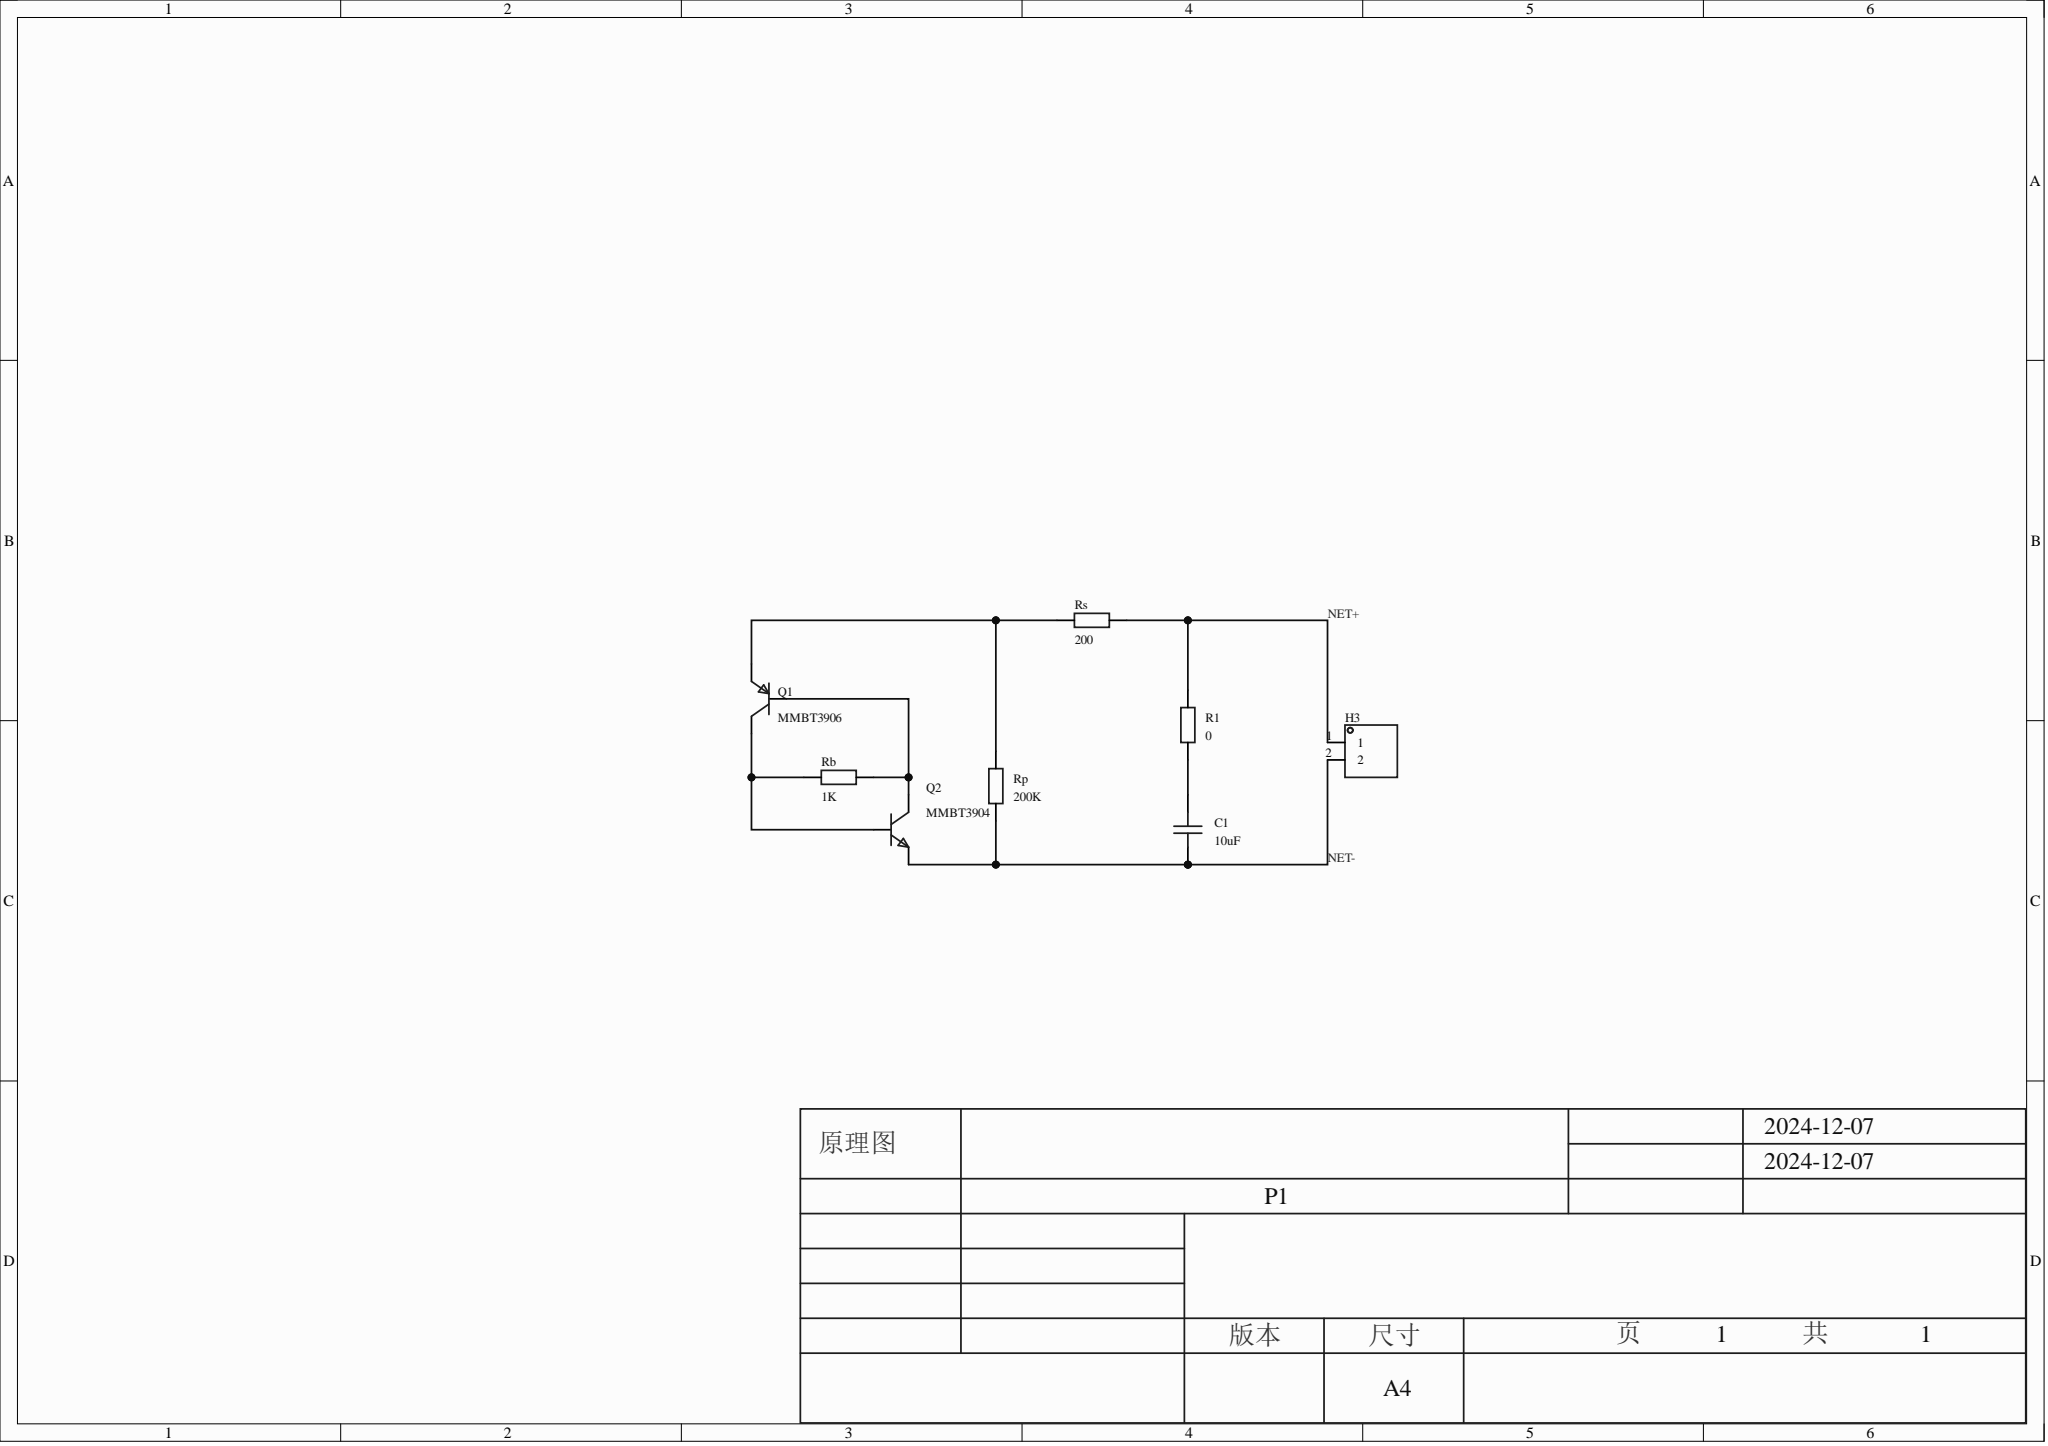Circuit board | Altium Designer | 8 parts | 6 nets
Bill of materials:
Comment,Description,Designator,Footprint,LibRef,Quantity
"10uF","","C1","C0402","CAP_0402","1"
"","","H3","HDR-TH_2P-P2.54-V-M-1","HDR-M_2.54_1x2P","1"
"MMBT3906","","Q1","SOT-23-3_L2.9-W1.3-P1.90-LS2.4-BR","MMBT3906_C18195368","1"
"MMBT3904","","Q2","SOT-23-3_L2.9-W1.3-P1.90-LS2.4-BR","MMBT3904","1"
"0","","R1","R0402","Res_0402","1"
"1K","","Rb","R0402","Res_0402","1"
"200K","","Rp","R0402","Res_0402","1"
"200","","Rs","R0402","Res_0402","1"
Netlist (Protel format):
[
C1
C0402
10uF



]
[
H3
HDR-TH_2P-P2.54-V-M-1




]
[
Q1
SOT-23-3_L2.9-W1.3-P1.90-LS2.4-BR
MMBT3906



]
[
Q2
SOT-23-3_L2.9-W1.3-P1.90-LS2.4-BR
MMBT3904



]
[
R1
R0402
0



]
[
Rb
R0402
1K



]
[
Rp
R0402
200K



]
[
Rs
R0402
200



]
(
NetQ1_3
Q1-3
Q2-1
Rb-1
)
(
NetQ1_2
Q1-2
Rp-2
Rs-1
)
(
NetQ1_1
Q1-1
Q2-3
Rb-2
)
(
NetC1_2
C1-2
R1-1
)
(
NET-
C1-1
H3-2
Q2-2
Rp-1
)
(
NET+
H3-1
R1-2
Rs-2
)